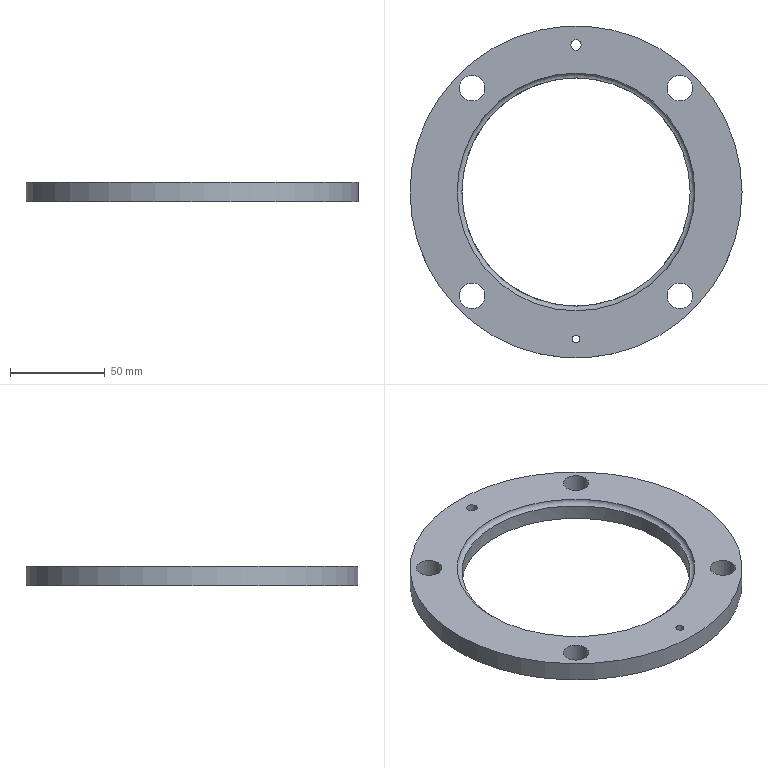Part | NX | features 2 2 | 1 solid | 12 faces | box 175 x 175 x 10.5 mm | volume 124846 mm3 | cylinder 8 | plane 2 | torus 1 | cone 1 | commonest cylinder face diameters 13.5 x4 4.2 x1 5.5 x1 120.3 x1 175 x1
STEP:
#1=CARTESIAN_POINT('',(2217.5,265.,29.5));
#2=VERTEX_POINT('',#1);
#3=CARTESIAN_POINT('',(2130.,265.,29.5));
#4=DIRECTION('',(0.,0.,1.));
#5=DIRECTION('',(1.,0.,0.));
#6=AXIS2_PLACEMENT_3D('',#3,#4,#5);
#7=CIRCLE('',#6,87.5);
#8=EDGE_CURVE('',#2,#2,#7,.T.);
#9=ORIENTED_EDGE('',*,*,#8,.F.);
#10=EDGE_LOOP('',(#9));
#11=FACE_BOUND('',#10,.T.);
#12=CARTESIAN_POINT('',(2217.5,265.,19.));
#13=VERTEX_POINT('',#12);
#14=CARTESIAN_POINT('',(2130.,265.,19.));
#15=DIRECTION('',(0.,0.,-1.));
#16=DIRECTION('',(1.,0.,0.));
#17=AXIS2_PLACEMENT_3D('',#14,#15,#16);
#18=CIRCLE('',#17,87.5);
#19=EDGE_CURVE('',#13,#13,#18,.T.);
#20=ORIENTED_EDGE('',*,*,#19,.F.);
#21=EDGE_LOOP('',(#20));
#22=FACE_BOUND('',#21,.T.);
#23=CARTESIAN_POINT('',(2130.,265.,29.5));
#24=DIRECTION('',(0.,0.,1.));
#25=DIRECTION('',(-1.,0.,0.));
#26=AXIS2_PLACEMENT_3D('',#23,#24,#25);
#27=CYLINDRICAL_SURFACE('',#26,87.5);
#28=ADVANCED_FACE('',(#11,#22),#27,.T.);
#29=CARTESIAN_POINT('',(2190.15,265.,27.));
#30=VERTEX_POINT('',#29);
#31=CARTESIAN_POINT('',(2130.,265.,27.));
#32=DIRECTION('',(0.,0.,-1.));
#33=DIRECTION('',(1.,0.,0.));
#34=AXIS2_PLACEMENT_3D('',#31,#32,#33);
#35=CIRCLE('',#34,60.15);
#36=EDGE_CURVE('',#30,#30,#35,.T.);
#37=ORIENTED_EDGE('',*,*,#36,.F.);
#38=EDGE_LOOP('',(#37));
#39=FACE_BOUND('',#38,.T.);
#40=CARTESIAN_POINT('',(2190.15,265.,19.));
#41=VERTEX_POINT('',#40);
#42=CARTESIAN_POINT('',(2130.,265.,19.));
#43=DIRECTION('',(0.,0.,-1.));
#44=DIRECTION('',(1.,0.,0.));
#45=AXIS2_PLACEMENT_3D('',#42,#43,#44);
#46=CIRCLE('',#45,60.15);
#47=EDGE_CURVE('',#41,#41,#46,.T.);
#48=ORIENTED_EDGE('',*,*,#47,.T.);
#49=EDGE_LOOP('',(#48));
#50=FACE_BOUND('',#49,.T.);
#51=CARTESIAN_POINT('',(2130.,265.,-2.));
#52=DIRECTION('',(0.,0.,-1.));
#53=DIRECTION('',(1.,0.,0.));
#54=AXIS2_PLACEMENT_3D('',#51,#52,#53);
#55=CYLINDRICAL_SURFACE('',#54,60.15);
#56=ADVANCED_FACE('',(#39,#50),#55,.F.);
#57=CARTESIAN_POINT('',(2082.,319.75,29.5));
#58=VERTEX_POINT('',#57);
#59=CARTESIAN_POINT('',(2075.25,319.75,29.5));
#60=DIRECTION('',(0.,0.,1.));
#61=DIRECTION('',(1.,0.,0.));
#62=AXIS2_PLACEMENT_3D('',#59,#60,#61);
#63=CIRCLE('',#62,6.75);
#64=EDGE_CURVE('',#58,#58,#63,.T.);
#65=ORIENTED_EDGE('',*,*,#64,.T.);
#66=EDGE_LOOP('',(#65));
#67=FACE_BOUND('',#66,.T.);
#68=CARTESIAN_POINT('',(2082.,319.75,19.));
#69=VERTEX_POINT('',#68);
#70=CARTESIAN_POINT('',(2075.25,319.75,19.));
#71=DIRECTION('',(0.,0.,-1.));
#72=DIRECTION('',(1.,0.,0.));
#73=AXIS2_PLACEMENT_3D('',#70,#71,#72);
#74=CIRCLE('',#73,6.75);
#75=EDGE_CURVE('',#69,#69,#74,.T.);
#76=ORIENTED_EDGE('',*,*,#75,.T.);
#77=EDGE_LOOP('',(#76));
#78=FACE_BOUND('',#77,.T.);
#79=CARTESIAN_POINT('',(2075.25,319.75,-2.));
#80=DIRECTION('',(0.,0.,-1.));
#81=DIRECTION('',(1.,0.,0.));
#82=AXIS2_PLACEMENT_3D('',#79,#80,#81);
#83=CYLINDRICAL_SURFACE('',#82,6.75);
#84=ADVANCED_FACE('',(#67,#78),#83,.F.);
#85=CARTESIAN_POINT('',(2082.,210.25,29.5));
#86=VERTEX_POINT('',#85);
#87=CARTESIAN_POINT('',(2075.25,210.25,29.5));
#88=DIRECTION('',(0.,0.,1.));
#89=DIRECTION('',(1.,0.,0.));
#90=AXIS2_PLACEMENT_3D('',#87,#88,#89);
#91=CIRCLE('',#90,6.75);
#92=EDGE_CURVE('',#86,#86,#91,.T.);
#93=ORIENTED_EDGE('',*,*,#92,.T.);
#94=EDGE_LOOP('',(#93));
#95=FACE_BOUND('',#94,.T.);
#96=CARTESIAN_POINT('',(2082.,210.25,19.));
#97=VERTEX_POINT('',#96);
#98=CARTESIAN_POINT('',(2075.25,210.25,19.));
#99=DIRECTION('',(0.,0.,-1.));
#100=DIRECTION('',(1.,0.,0.));
#101=AXIS2_PLACEMENT_3D('',#98,#99,#100);
#102=CIRCLE('',#101,6.75);
#103=EDGE_CURVE('',#97,#97,#102,.T.);
#104=ORIENTED_EDGE('',*,*,#103,.T.);
#105=EDGE_LOOP('',(#104));
#106=FACE_BOUND('',#105,.T.);
#107=CARTESIAN_POINT('',(2075.25,210.25,-2.));
#108=DIRECTION('',(0.,0.,-1.));
#109=DIRECTION('',(1.,0.,0.));
#110=AXIS2_PLACEMENT_3D('',#107,#108,#109);
#111=CYLINDRICAL_SURFACE('',#110,6.75);
#112=ADVANCED_FACE('',(#95,#106),#111,.F.);
#113=CARTESIAN_POINT('',(2191.5,319.75,29.5));
#114=VERTEX_POINT('',#113);
#115=CARTESIAN_POINT('',(2184.75,319.75,29.5));
#116=DIRECTION('',(0.,0.,1.));
#117=DIRECTION('',(1.,0.,0.));
#118=AXIS2_PLACEMENT_3D('',#115,#116,#117);
#119=CIRCLE('',#118,6.75);
#120=EDGE_CURVE('',#114,#114,#119,.T.);
#121=ORIENTED_EDGE('',*,*,#120,.T.);
#122=EDGE_LOOP('',(#121));
#123=FACE_BOUND('',#122,.T.);
#124=CARTESIAN_POINT('',(2191.5,319.75,19.));
#125=VERTEX_POINT('',#124);
#126=CARTESIAN_POINT('',(2184.75,319.75,19.));
#127=DIRECTION('',(0.,0.,-1.));
#128=DIRECTION('',(1.,0.,0.));
#129=AXIS2_PLACEMENT_3D('',#126,#127,#128);
#130=CIRCLE('',#129,6.75);
#131=EDGE_CURVE('',#125,#125,#130,.T.);
#132=ORIENTED_EDGE('',*,*,#131,.T.);
#133=EDGE_LOOP('',(#132));
#134=FACE_BOUND('',#133,.T.);
#135=CARTESIAN_POINT('',(2184.75,319.75,-2.));
#136=DIRECTION('',(0.,0.,-1.));
#137=DIRECTION('',(1.,0.,0.));
#138=AXIS2_PLACEMENT_3D('',#135,#136,#137);
#139=CYLINDRICAL_SURFACE('',#138,6.75);
#140=ADVANCED_FACE('',(#123,#134),#139,.F.);
#141=CARTESIAN_POINT('',(2191.5,210.25,29.5));
#142=VERTEX_POINT('',#141);
#143=CARTESIAN_POINT('',(2184.75,210.25,29.5));
#144=DIRECTION('',(0.,0.,1.));
#145=DIRECTION('',(1.,0.,0.));
#146=AXIS2_PLACEMENT_3D('',#143,#144,#145);
#147=CIRCLE('',#146,6.75);
#148=EDGE_CURVE('',#142,#142,#147,.T.);
#149=ORIENTED_EDGE('',*,*,#148,.T.);
#150=EDGE_LOOP('',(#149));
#151=FACE_BOUND('',#150,.T.);
#152=CARTESIAN_POINT('',(2191.5,210.25,19.));
#153=VERTEX_POINT('',#152);
#154=CARTESIAN_POINT('',(2184.75,210.25,19.));
#155=DIRECTION('',(0.,0.,-1.));
#156=DIRECTION('',(1.,0.,0.));
#157=AXIS2_PLACEMENT_3D('',#154,#155,#156);
#158=CIRCLE('',#157,6.75);
#159=EDGE_CURVE('',#153,#153,#158,.T.);
#160=ORIENTED_EDGE('',*,*,#159,.T.);
#161=EDGE_LOOP('',(#160));
#162=FACE_BOUND('',#161,.T.);
#163=CARTESIAN_POINT('',(2184.75,210.25,-2.));
#164=DIRECTION('',(0.,0.,-1.));
#165=DIRECTION('',(1.,0.,0.));
#166=AXIS2_PLACEMENT_3D('',#163,#164,#165);
#167=CYLINDRICAL_SURFACE('',#166,6.75);
#168=ADVANCED_FACE('',(#151,#162),#167,.F.);
#169=CARTESIAN_POINT('',(2067.35,265.,29.5));
#170=VERTEX_POINT('',#169);
#171=CARTESIAN_POINT('',(2130.,265.,29.5));
#172=DIRECTION('',(0.,0.,1.));
#173=DIRECTION('',(-1.,0.,0.));
#174=AXIS2_PLACEMENT_3D('',#171,#172,#173);
#175=CIRCLE('',#174,62.65);
#176=EDGE_CURVE('',#170,#170,#175,.T.);
#177=ORIENTED_EDGE('',*,*,#176,.T.);
#178=EDGE_LOOP('',(#177));
#179=FACE_BOUND('',#178,.T.);
#180=ORIENTED_EDGE('',*,*,#36,.T.);
#181=EDGE_LOOP('',(#180));
#182=FACE_BOUND('',#181,.T.);
#183=CARTESIAN_POINT('',(2130.,265.,29.5));
#184=DIRECTION('',(0.,0.,1.));
#185=DIRECTION('',(-1.,0.,0.));
#186=AXIS2_PLACEMENT_3D('',#183,#184,#185);
#187=TOROIDAL_SURFACE('',#186,60.15,2.5);
#188=ADVANCED_FACE('',(#179,#182),#187,.F.);
#189=CARTESIAN_POINT('',(2130.,347.7,19.));
#190=VERTEX_POINT('',#189);
#191=CARTESIAN_POINT('',(2130.,342.5,19.));
#192=DIRECTION('',(0.,0.,-1.));
#193=DIRECTION('',(0.,1.,0.));
#194=AXIS2_PLACEMENT_3D('',#191,#192,#193);
#195=CIRCLE('',#194,5.2);
#196=EDGE_CURVE('',#190,#190,#195,.T.);
#197=ORIENTED_EDGE('',*,*,#196,.T.);
#198=EDGE_LOOP('',(#197));
#199=FACE_BOUND('',#198,.T.);
#200=CARTESIAN_POINT('',(2130.,345.25,21.45));
#201=VERTEX_POINT('',#200);
#202=CARTESIAN_POINT('',(2130.,342.5,21.45));
#203=DIRECTION('',(0.,0.,1.));
#204=DIRECTION('',(0.,1.,0.));
#205=AXIS2_PLACEMENT_3D('',#202,#203,#204);
#206=CIRCLE('',#205,2.75);
#207=EDGE_CURVE('',#201,#201,#206,.T.);
#208=ORIENTED_EDGE('',*,*,#207,.T.);
#209=EDGE_LOOP('',(#208));
#210=FACE_BOUND('',#209,.T.);
#211=CARTESIAN_POINT('',(2130.,342.5,20.225));
#212=DIRECTION('',(0.,0.,-1.));
#213=DIRECTION('',(1.,0.,0.));
#214=AXIS2_PLACEMENT_3D('',#211,#212,#213);
#215=CONICAL_SURFACE('',#214,3.975,0.7854);
#216=ADVANCED_FACE('',(#199,#210),#215,.F.);
#217=ORIENTED_EDGE('',*,*,#207,.F.);
#218=EDGE_LOOP('',(#217));
#219=FACE_BOUND('',#218,.T.);
#220=CARTESIAN_POINT('',(2130.,345.25,29.5));
#221=VERTEX_POINT('',#220);
#222=CARTESIAN_POINT('',(2130.,342.5,29.5));
#223=DIRECTION('',(0.,0.,1.));
#224=DIRECTION('',(0.,1.,0.));
#225=AXIS2_PLACEMENT_3D('',#222,#223,#224);
#226=CIRCLE('',#225,2.75);
#227=EDGE_CURVE('',#221,#221,#226,.T.);
#228=ORIENTED_EDGE('',*,*,#227,.T.);
#229=EDGE_LOOP('',(#228));
#230=FACE_BOUND('',#229,.T.);
#231=CARTESIAN_POINT('',(2130.,342.5,25.475));
#232=DIRECTION('',(0.,0.,1.));
#233=DIRECTION('',(-1.,0.,0.));
#234=AXIS2_PLACEMENT_3D('',#231,#232,#233);
#235=CYLINDRICAL_SURFACE('',#234,2.75);
#236=ADVANCED_FACE('',(#219,#230),#235,.F.);
#237=CARTESIAN_POINT('',(2130.,185.4,29.5));
#238=VERTEX_POINT('',#237);
#239=CARTESIAN_POINT('',(2130.,187.5,29.5));
#240=DIRECTION('',(0.,0.,1.));
#241=DIRECTION('',(0.,-1.,0.));
#242=AXIS2_PLACEMENT_3D('',#239,#240,#241);
#243=CIRCLE('',#242,2.1);
#244=EDGE_CURVE('',#238,#238,#243,.T.);
#245=ORIENTED_EDGE('',*,*,#244,.T.);
#246=EDGE_LOOP('',(#245));
#247=FACE_BOUND('',#246,.T.);
#248=CARTESIAN_POINT('',(2130.,185.4,19.));
#249=VERTEX_POINT('',#248);
#250=CARTESIAN_POINT('',(2130.,187.5,19.));
#251=DIRECTION('',(0.,0.,-1.));
#252=DIRECTION('',(0.,-1.,0.));
#253=AXIS2_PLACEMENT_3D('',#250,#251,#252);
#254=CIRCLE('',#253,2.1);
#255=EDGE_CURVE('',#249,#249,#254,.T.);
#256=ORIENTED_EDGE('',*,*,#255,.T.);
#257=EDGE_LOOP('',(#256));
#258=FACE_BOUND('',#257,.T.);
#259=CARTESIAN_POINT('',(2130.,187.5,24.25));
#260=DIRECTION('',(0.,0.,-1.));
#261=DIRECTION('',(1.,0.,0.));
#262=AXIS2_PLACEMENT_3D('',#259,#260,#261);
#263=CYLINDRICAL_SURFACE('',#262,2.1);
#264=ADVANCED_FACE('',(#247,#258),#263,.F.);
#265=ORIENTED_EDGE('',*,*,#255,.F.);
#266=EDGE_LOOP('',(#265));
#267=FACE_BOUND('',#266,.T.);
#268=ORIENTED_EDGE('',*,*,#196,.F.);
#269=EDGE_LOOP('',(#268));
#270=FACE_BOUND('',#269,.T.);
#271=ORIENTED_EDGE('',*,*,#159,.F.);
#272=EDGE_LOOP('',(#271));
#273=FACE_BOUND('',#272,.T.);
#274=ORIENTED_EDGE('',*,*,#131,.F.);
#275=EDGE_LOOP('',(#274));
#276=FACE_BOUND('',#275,.T.);
#277=ORIENTED_EDGE('',*,*,#103,.F.);
#278=EDGE_LOOP('',(#277));
#279=FACE_BOUND('',#278,.T.);
#280=ORIENTED_EDGE('',*,*,#75,.F.);
#281=EDGE_LOOP('',(#280));
#282=FACE_BOUND('',#281,.T.);
#283=ORIENTED_EDGE('',*,*,#47,.F.);
#284=EDGE_LOOP('',(#283));
#285=FACE_BOUND('',#284,.T.);
#286=ORIENTED_EDGE('',*,*,#19,.T.);
#287=EDGE_LOOP('',(#286));
#288=FACE_BOUND('',#287,.T.);
#289=CARTESIAN_POINT('',(2130.,265.,19.));
#290=DIRECTION('',(0.,0.,-1.));
#291=DIRECTION('',(1.,0.,0.));
#292=AXIS2_PLACEMENT_3D('',#289,#290,#291);
#293=PLANE('',#292);
#294=ADVANCED_FACE('',(#267,#270,#273,#276,#279,#282,#285,#288),#293,.T.);
#295=ORIENTED_EDGE('',*,*,#244,.F.);
#296=EDGE_LOOP('',(#295));
#297=FACE_BOUND('',#296,.T.);
#298=ORIENTED_EDGE('',*,*,#227,.F.);
#299=EDGE_LOOP('',(#298));
#300=FACE_BOUND('',#299,.T.);
#301=ORIENTED_EDGE('',*,*,#176,.F.);
#302=EDGE_LOOP('',(#301));
#303=FACE_BOUND('',#302,.T.);
#304=ORIENTED_EDGE('',*,*,#148,.F.);
#305=EDGE_LOOP('',(#304));
#306=FACE_BOUND('',#305,.T.);
#307=ORIENTED_EDGE('',*,*,#120,.F.);
#308=EDGE_LOOP('',(#307));
#309=FACE_BOUND('',#308,.T.);
#310=ORIENTED_EDGE('',*,*,#92,.F.);
#311=EDGE_LOOP('',(#310));
#312=FACE_BOUND('',#311,.T.);
#313=ORIENTED_EDGE('',*,*,#64,.F.);
#314=EDGE_LOOP('',(#313));
#315=FACE_BOUND('',#314,.T.);
#316=ORIENTED_EDGE('',*,*,#8,.T.);
#317=EDGE_LOOP('',(#316));
#318=FACE_BOUND('',#317,.T.);
#319=CARTESIAN_POINT('',(2130.,265.,29.5));
#320=DIRECTION('',(0.,0.,-1.));
#321=DIRECTION('',(1.,0.,0.));
#322=AXIS2_PLACEMENT_3D('',#319,#320,#321);
#323=PLANE('',#322);
#324=ADVANCED_FACE('',(#297,#300,#303,#306,#309,#312,#315,#318),#323,.F.);
#325=CLOSED_SHELL('',(#28,#56,#84,#112,#140,#168,#188,#216,#236,#264,#294,#324));
#326=MANIFOLD_SOLID_BREP('',#325);
#327=(LENGTH_UNIT()NAMED_UNIT(*)SI_UNIT(.MILLI.,.METRE.));
#328=UNCERTAINTY_MEASURE_WITH_UNIT(LENGTH_MEASURE(0.00001),#327,'','');
#329=(NAMED_UNIT(*)PLANE_ANGLE_UNIT()SI_UNIT($,.RADIAN.));
#330=(NAMED_UNIT(*)SI_UNIT($,.STERADIAN.)SOLID_ANGLE_UNIT());
#331=(GEOMETRIC_REPRESENTATION_CONTEXT(3)GLOBAL_UNCERTAINTY_ASSIGNED_CONTEXT((#328))GLOBAL_UNIT_ASSIGNED_CONTEXT((#327,#329,#330))REPRESENTATION_CONTEXT('',''));
#332=ADVANCED_BREP_SHAPE_REPRESENTATION('',(#326),#331);